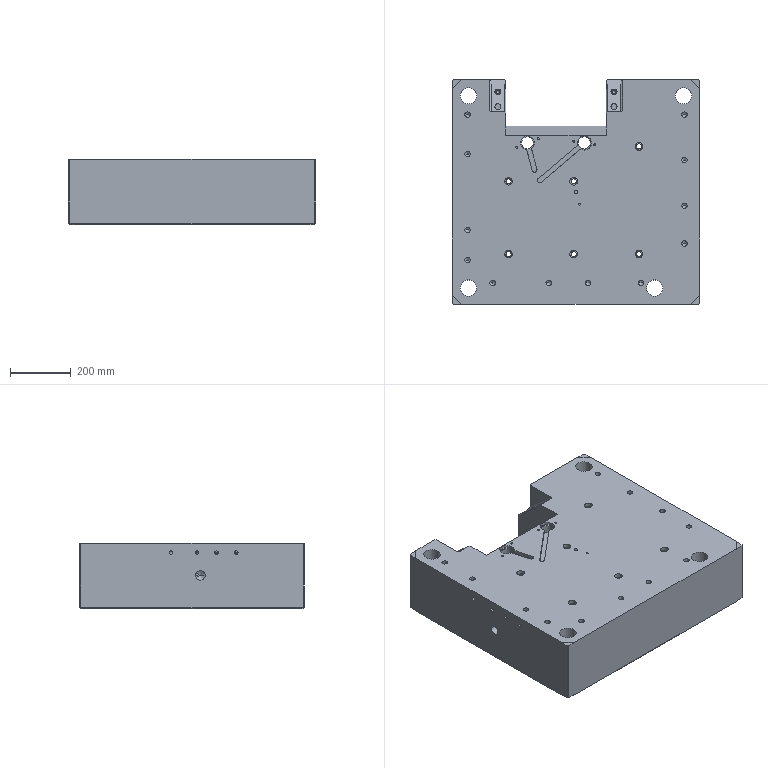Part | Creo | 1 solid | 743 faces | box 815 x 740 x 216 mm | volume 78173902 mm3 | plane 323 | cylinder 297 | cone 103 | spline 18 | other 2 | commonest cylinder face diameters 12 x37 5 x24 17.97 x24 16 x18 16.5 x16 22.5 x16